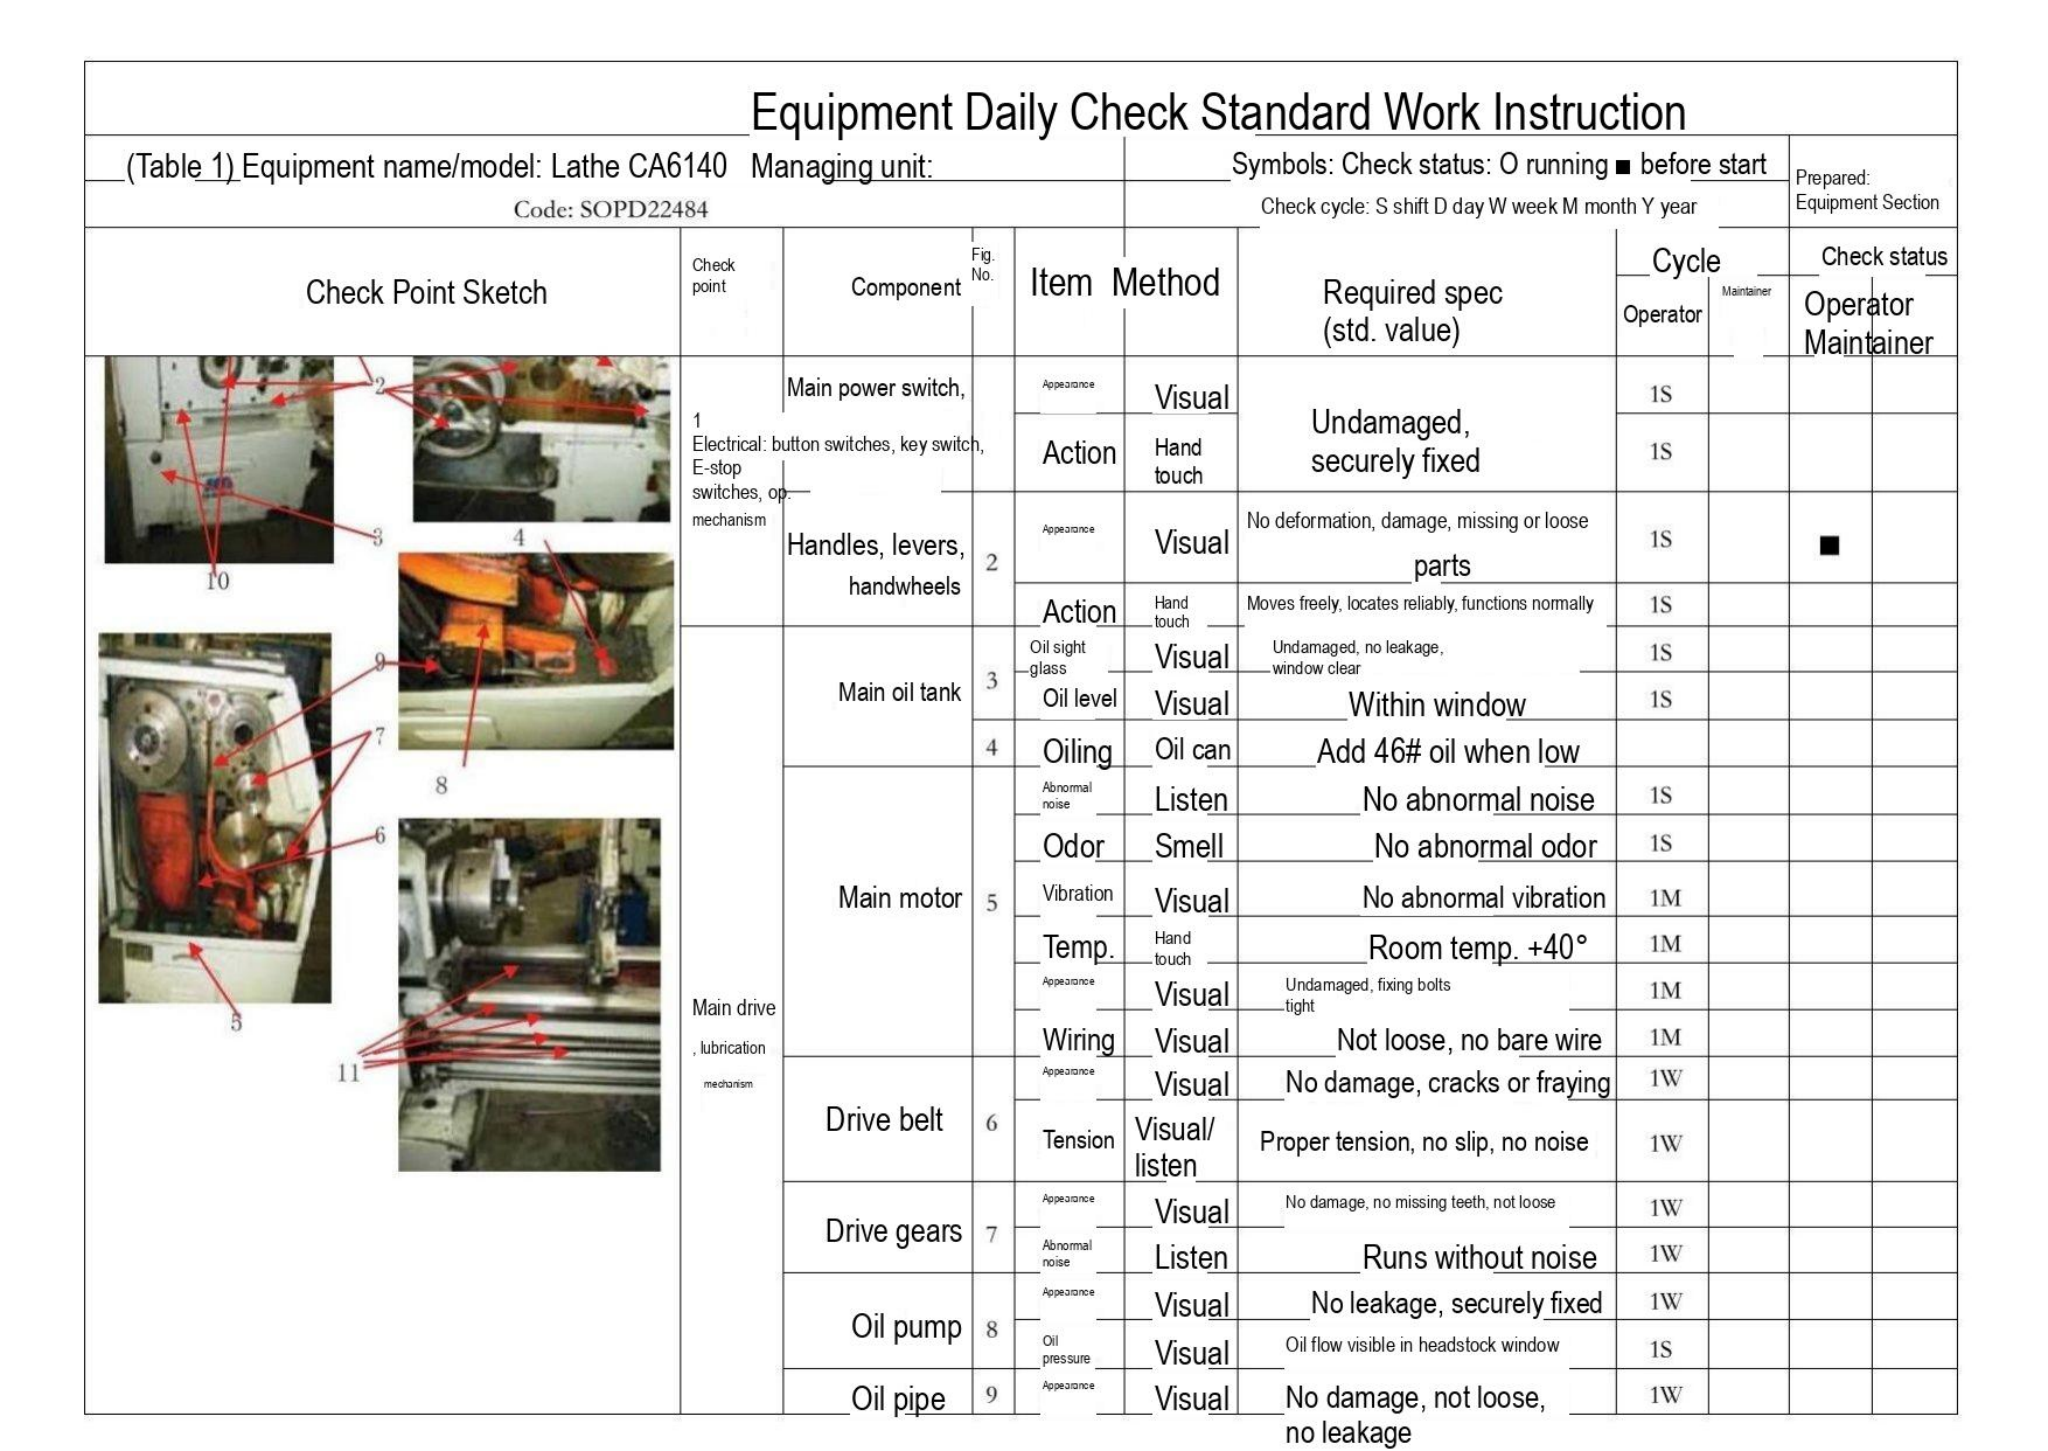# Equipment Daily Check Standard Work Instruction

(Table 1) Equipment name/model: Lathe CA6140 Managing unit:

Code: SOPD22484

Symbols: Check status: O running ■ before start

Check cycle: S shift D day W week M month Y year

Prepared: Equipment Section

Check Point Sketch

2 4 3 10 9 7 8 6 5 11

| Check point | Component | Fig. No. | Item | Method | Required spec (std. value) | Cycle Operator | Cycle Maintainer | Check status Operator | Check status Maintainer |
|---|---|---|---|---|---|---|---|---|---|
| 1 Electrical: button switches, key switch, E-stop switches, op. mechanism | Main power switch, | | Appearance | Visual | Undamaged, securely fixed | 1S | | | |
| | | | Action | Hand touch | | 1S | | | |
| | Handles, levers, handwheels | 2 | Appearance | Visual | No deformation, damage, missing or loose parts | 1S | | ■ | |
| | | | Action | Hand touch | Moves freely, locates reliably, functions normally | 1S | | | |
| Main drive, lubrication mechanism | Main oil tank | 3 | Oil sight glass | Visual | Undamaged, no leakage, window clear | 1S | | | |
| | | | Oil level | Visual | Within window | 1S | | | |
| | | 4 | Oiling | Oil can | Add 46# oil when low | | | | |
| | Main motor | 5 | Abnormal noise | Listen | No abnormal noise | 1S | | | |
| | | | Odor | Smell | No abnormal odor | 1S | | | |
| | | | Vibration | Visual | No abnormal vibration | 1M | | | |
| | | | Temp. | Hand touch | Room temp. +40° | 1M | | | |
| | | | Appearance | Visual | Undamaged, fixing bolts tight | 1M | | | |
| | | | Wiring | Visual | Not loose, no bare wire | 1M | | | |
| | Drive belt | 6 | Appearance | Visual | No damage, cracks or fraying | 1W | | | |
| | | | Tension | Visual/ listen | Proper tension, no slip, no noise | 1W | | | |
| | Drive gears | 7 | Appearance | Visual | No damage, no missing teeth, not loose | 1W | | | |
| | | | Abnormal noise | Listen | Runs without noise | 1W | | | |
| | Oil pump | 8 | Appearance | Visual | No leakage, securely fixed | 1W | | | |
| | | | Oil pressure | Visual | Oil flow visible in headstock window | 1S | | | |
| | Oil pipe | 9 | Appearance | Visual | No damage, not loose, no leakage | 1W | | | |
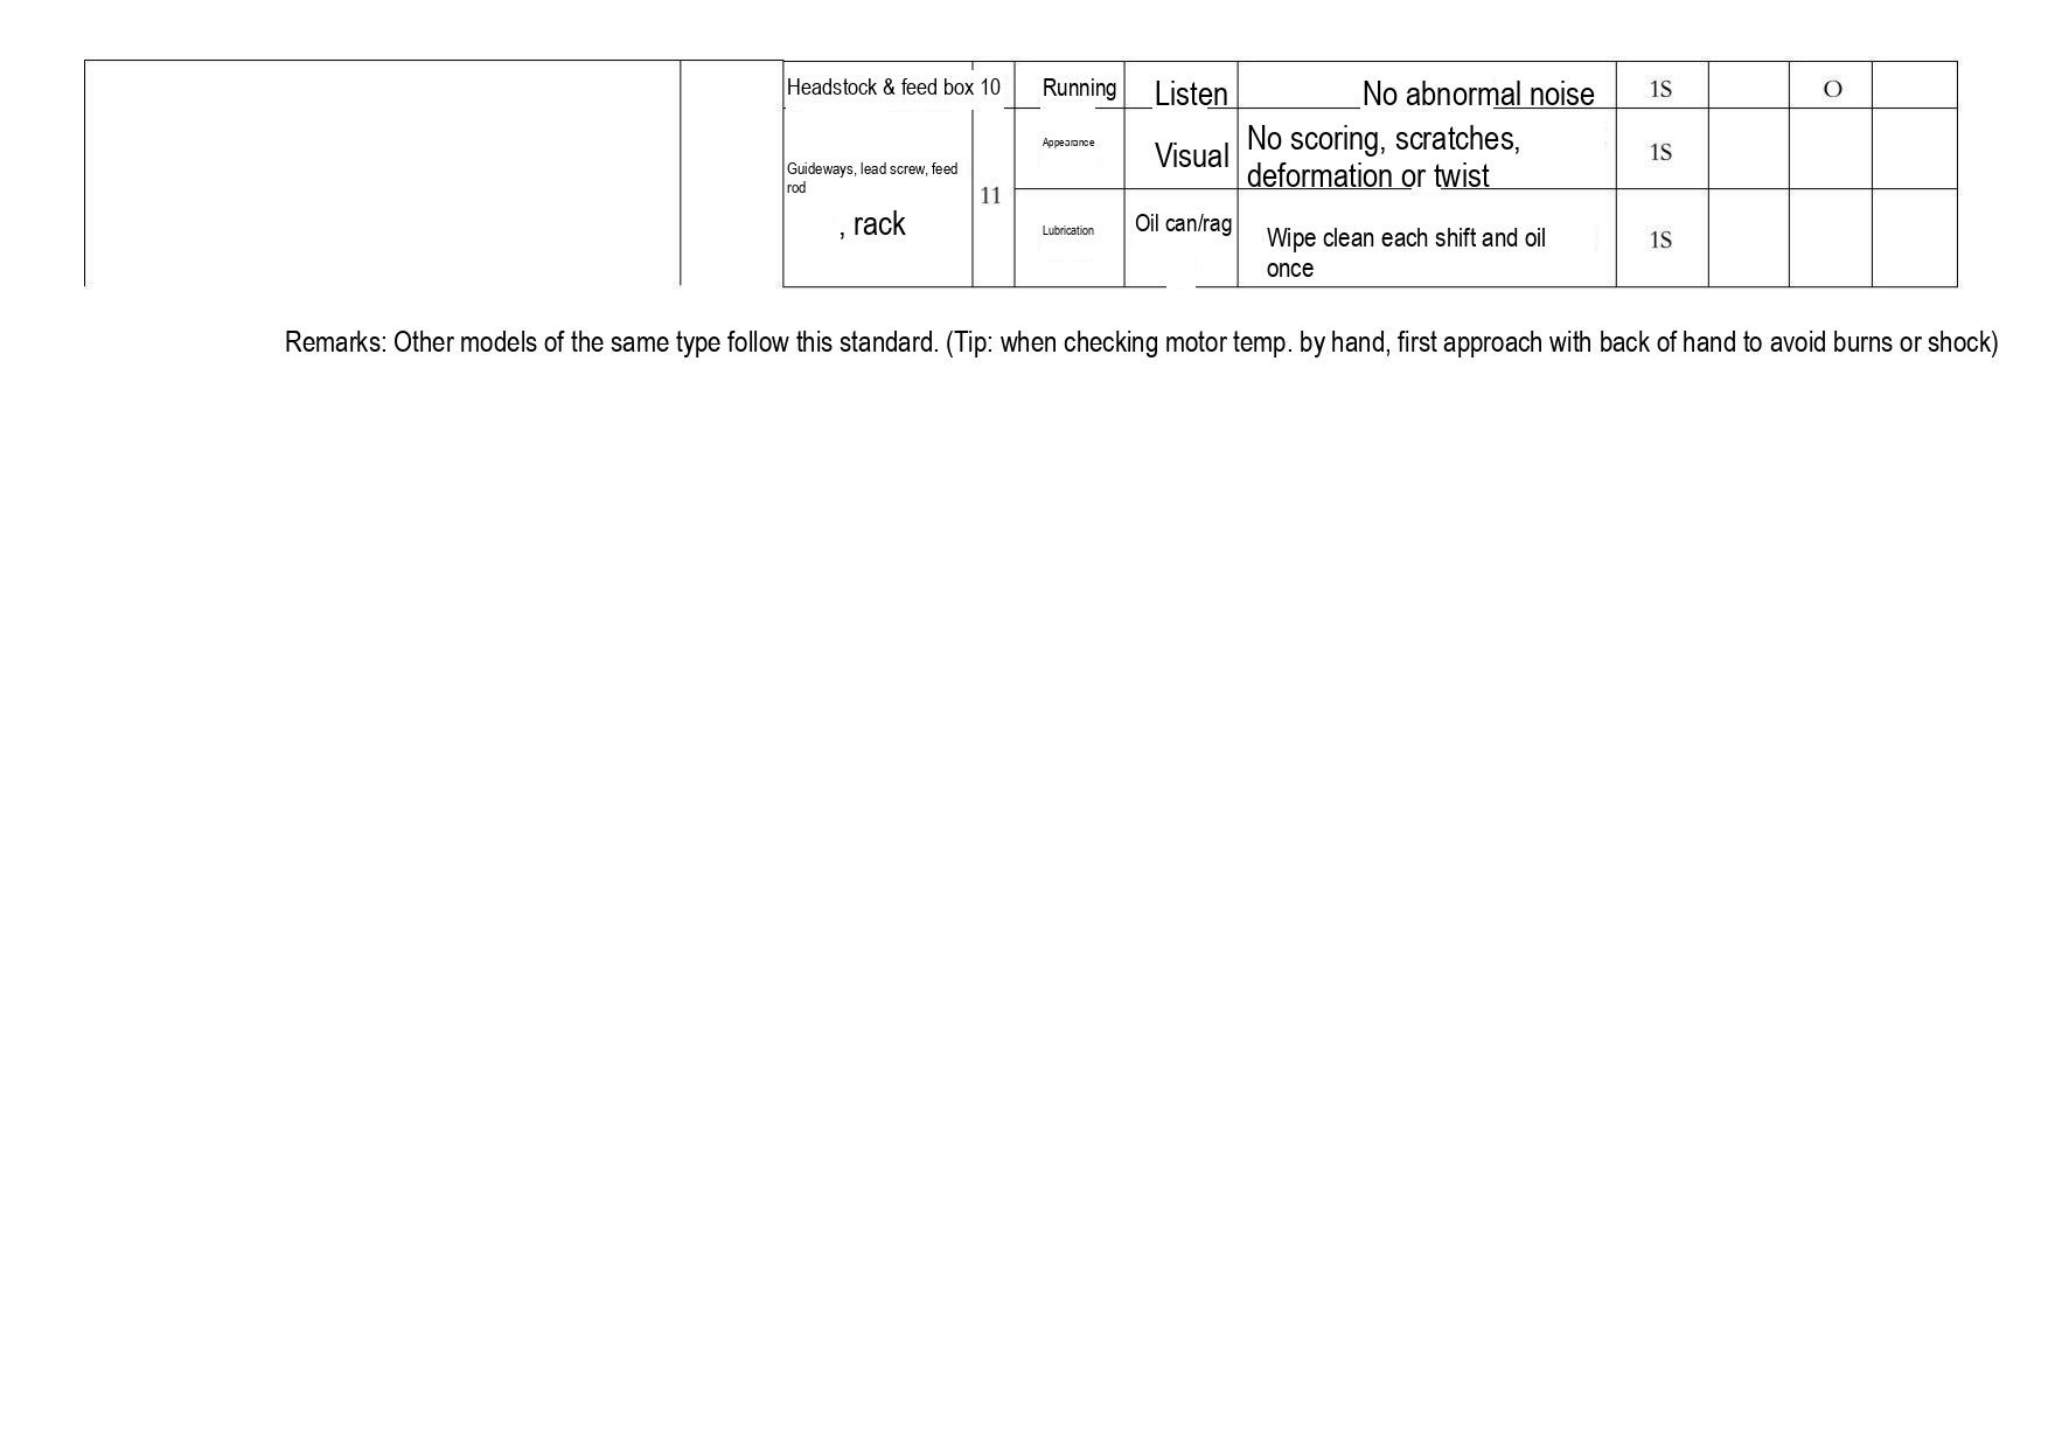| | | | | | | | | | | |
|---|---|---|---|---|---|---|---|---|---|---|
| | | Headstock & feed box | 10 | Running | Listen | No abnormal noise | 1S | | O | |
| | | Guideways, lead screw, feed rod , rack | 11 | Appearance | Visual | No scoring, scratches, deformation or twist | 1S | | | |
| | | | | Lubrication | Oil can/rag | Wipe clean each shift and oil once | 1S | | | |

Remarks: Other models of the same type follow this standard. (Tip: when checking motor temp. by hand, first approach with back of hand to avoid burns or shock)
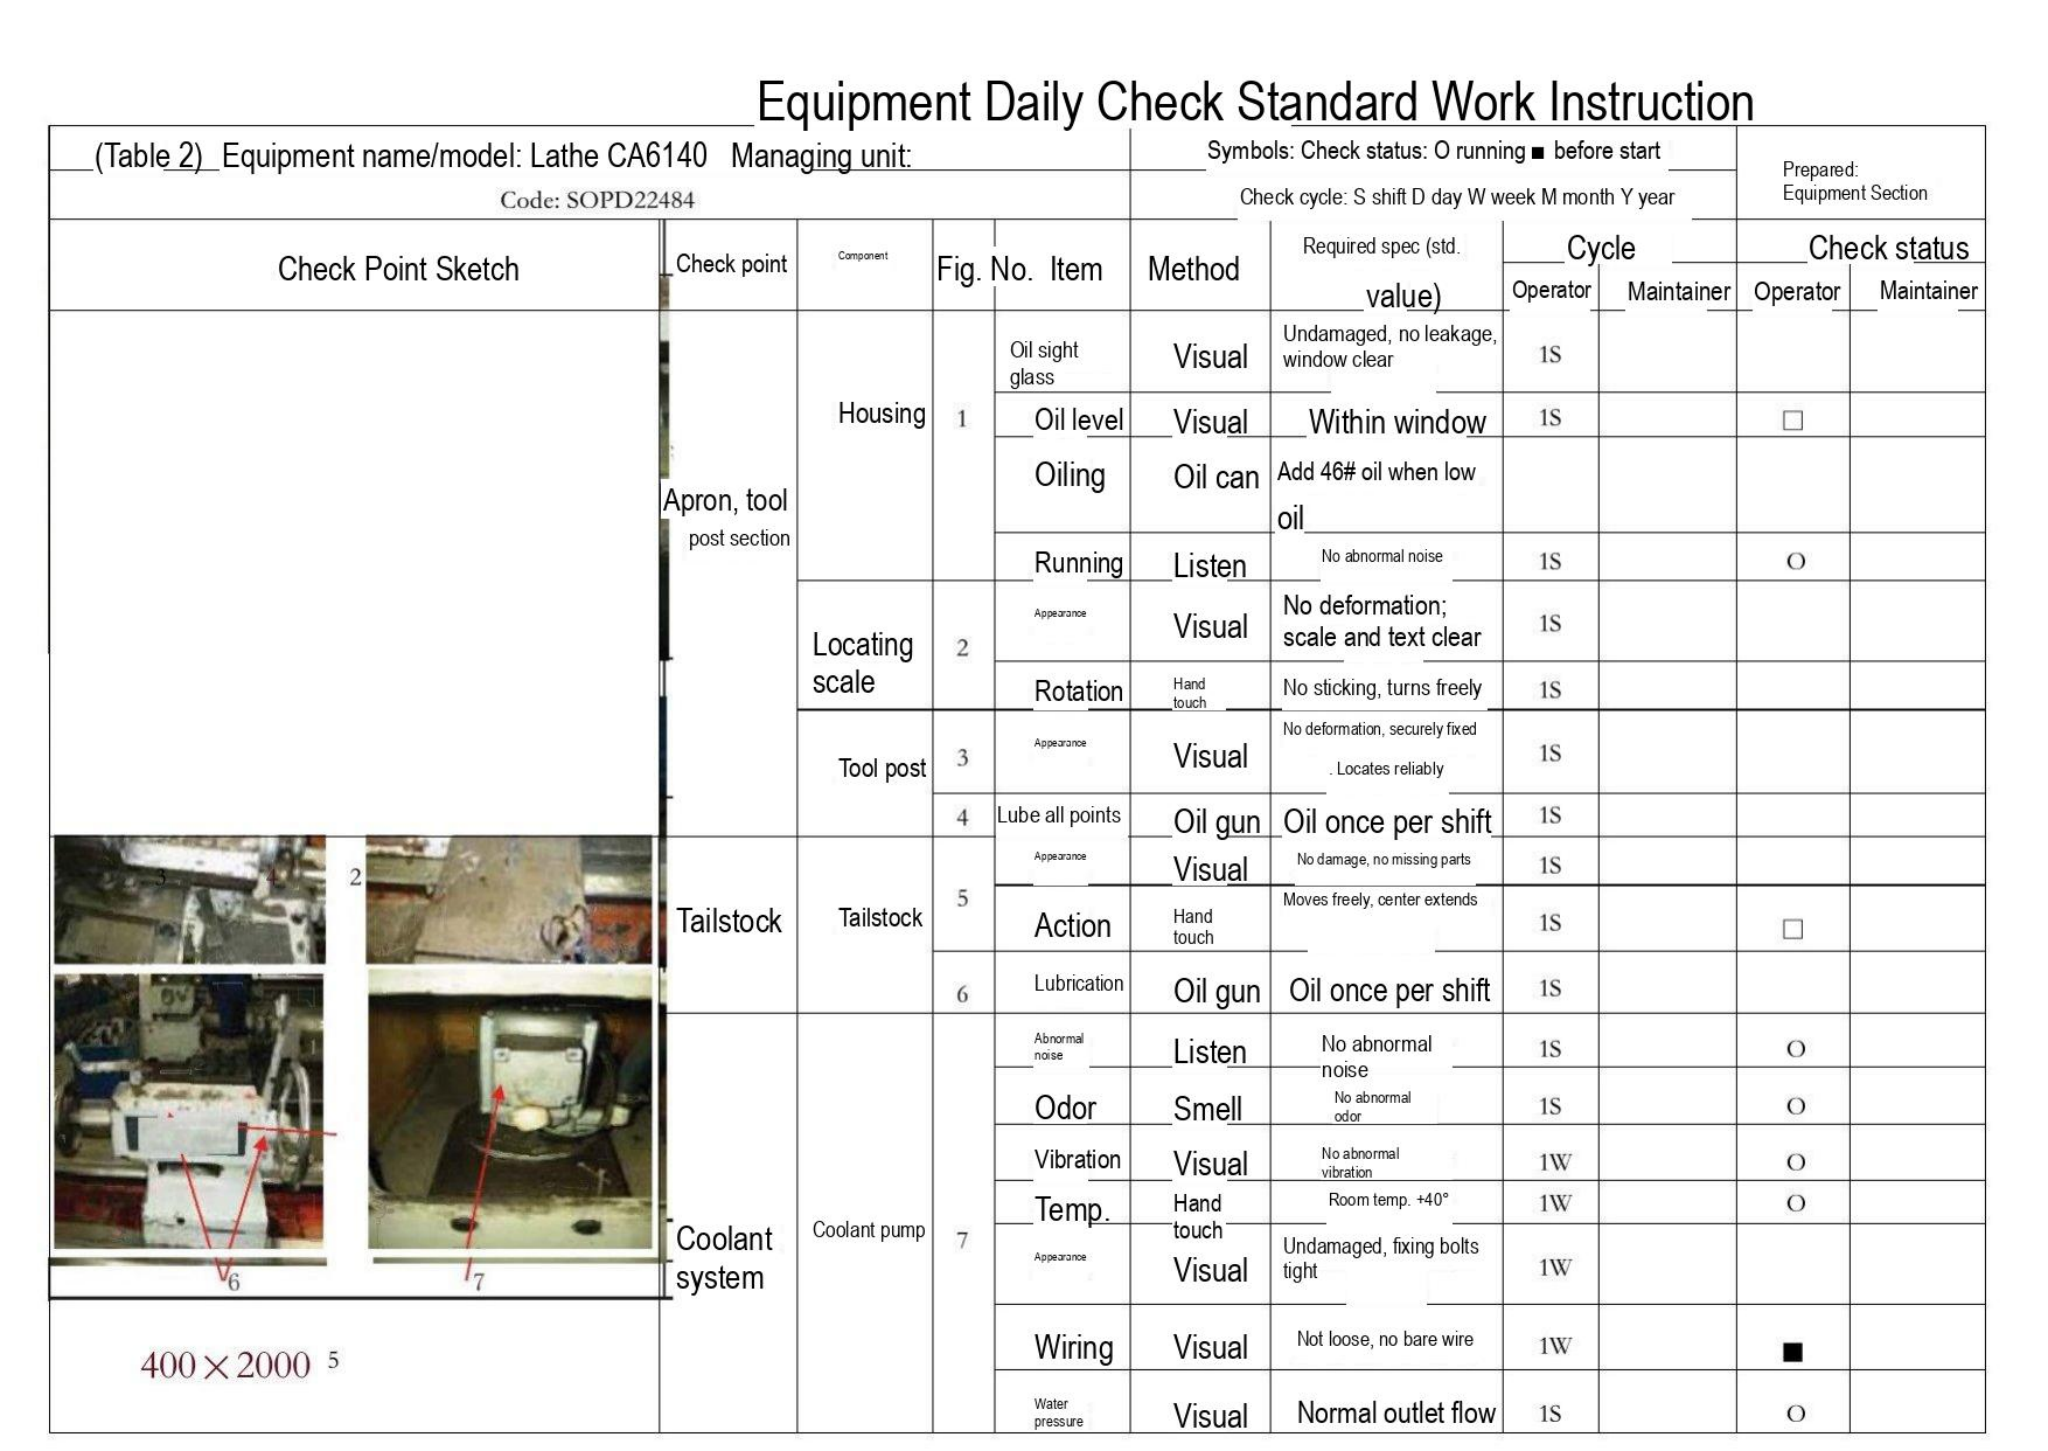# Equipment Daily Check Standard Work Instruction

(Table 2) Equipment name/model: Lathe CA6140 Managing unit:

Code: SOPD22484

Symbols: Check status: O running ■ before start

Check cycle: S shift D day W week M month Y year

Prepared: Equipment Section

Check Point Sketch

3 4 2

6 7

400 × 2000 5

| Check point | Component | Fig. No. | Item | Method | Required spec (std. value) | Cycle: Operator | Cycle: Maintainer | Check status: Operator | Check status: Maintainer |
|---|---|---|---|---|---|---|---|---|---|
| Apron, tool post section | Housing | 1 | Oil sight glass | Visual | Undamaged, no leakage, window clear | 1S | | | |
| | | | Oil level | Visual | Within window | 1S | | □ | |
| | | | Oiling | Oil can | Add 46# oil when low oil | | | | |
| | | | Running | Listen | No abnormal noise | 1S | | O | |
| | Locating scale | 2 | Appearance | Visual | No deformation; scale and text clear | 1S | | | |
| | | | Rotation | Hand touch | No sticking, turns freely | 1S | | | |
| | Tool post | 3 | Appearance | Visual | No deformation, securely fixed . Locates reliably | 1S | | | |
| | | 4 | Lube all points | Oil gun | Oil once per shift | 1S | | | |
| Tailstock | Tailstock | 5 | Appearance | Visual | No damage, no missing parts | 1S | | | |
| | | | Action | Hand touch | Moves freely, center extends | 1S | | □ | |
| | | 6 | Lubrication | Oil gun | Oil once per shift | 1S | | | |
| Coolant system | Coolant pump | 7 | Abnormal noise | Listen | No abnormal noise | 1S | | O | |
| | | | Odor | Smell | No abnormal odor | 1S | | O | |
| | | | Vibration | Visual | No abnormal vibration | 1W | | O | |
| | | | Temp. | Hand touch | Room temp. +40° | 1W | | O | |
| | | | Appearance | Visual | Undamaged, fixing bolts tight | 1W | | | |
| | | | Wiring | Visual | Not loose, no bare wire | 1W | | ■ | |
| | | | Water pressure | Visual | Normal outlet flow | 1S | | O | |
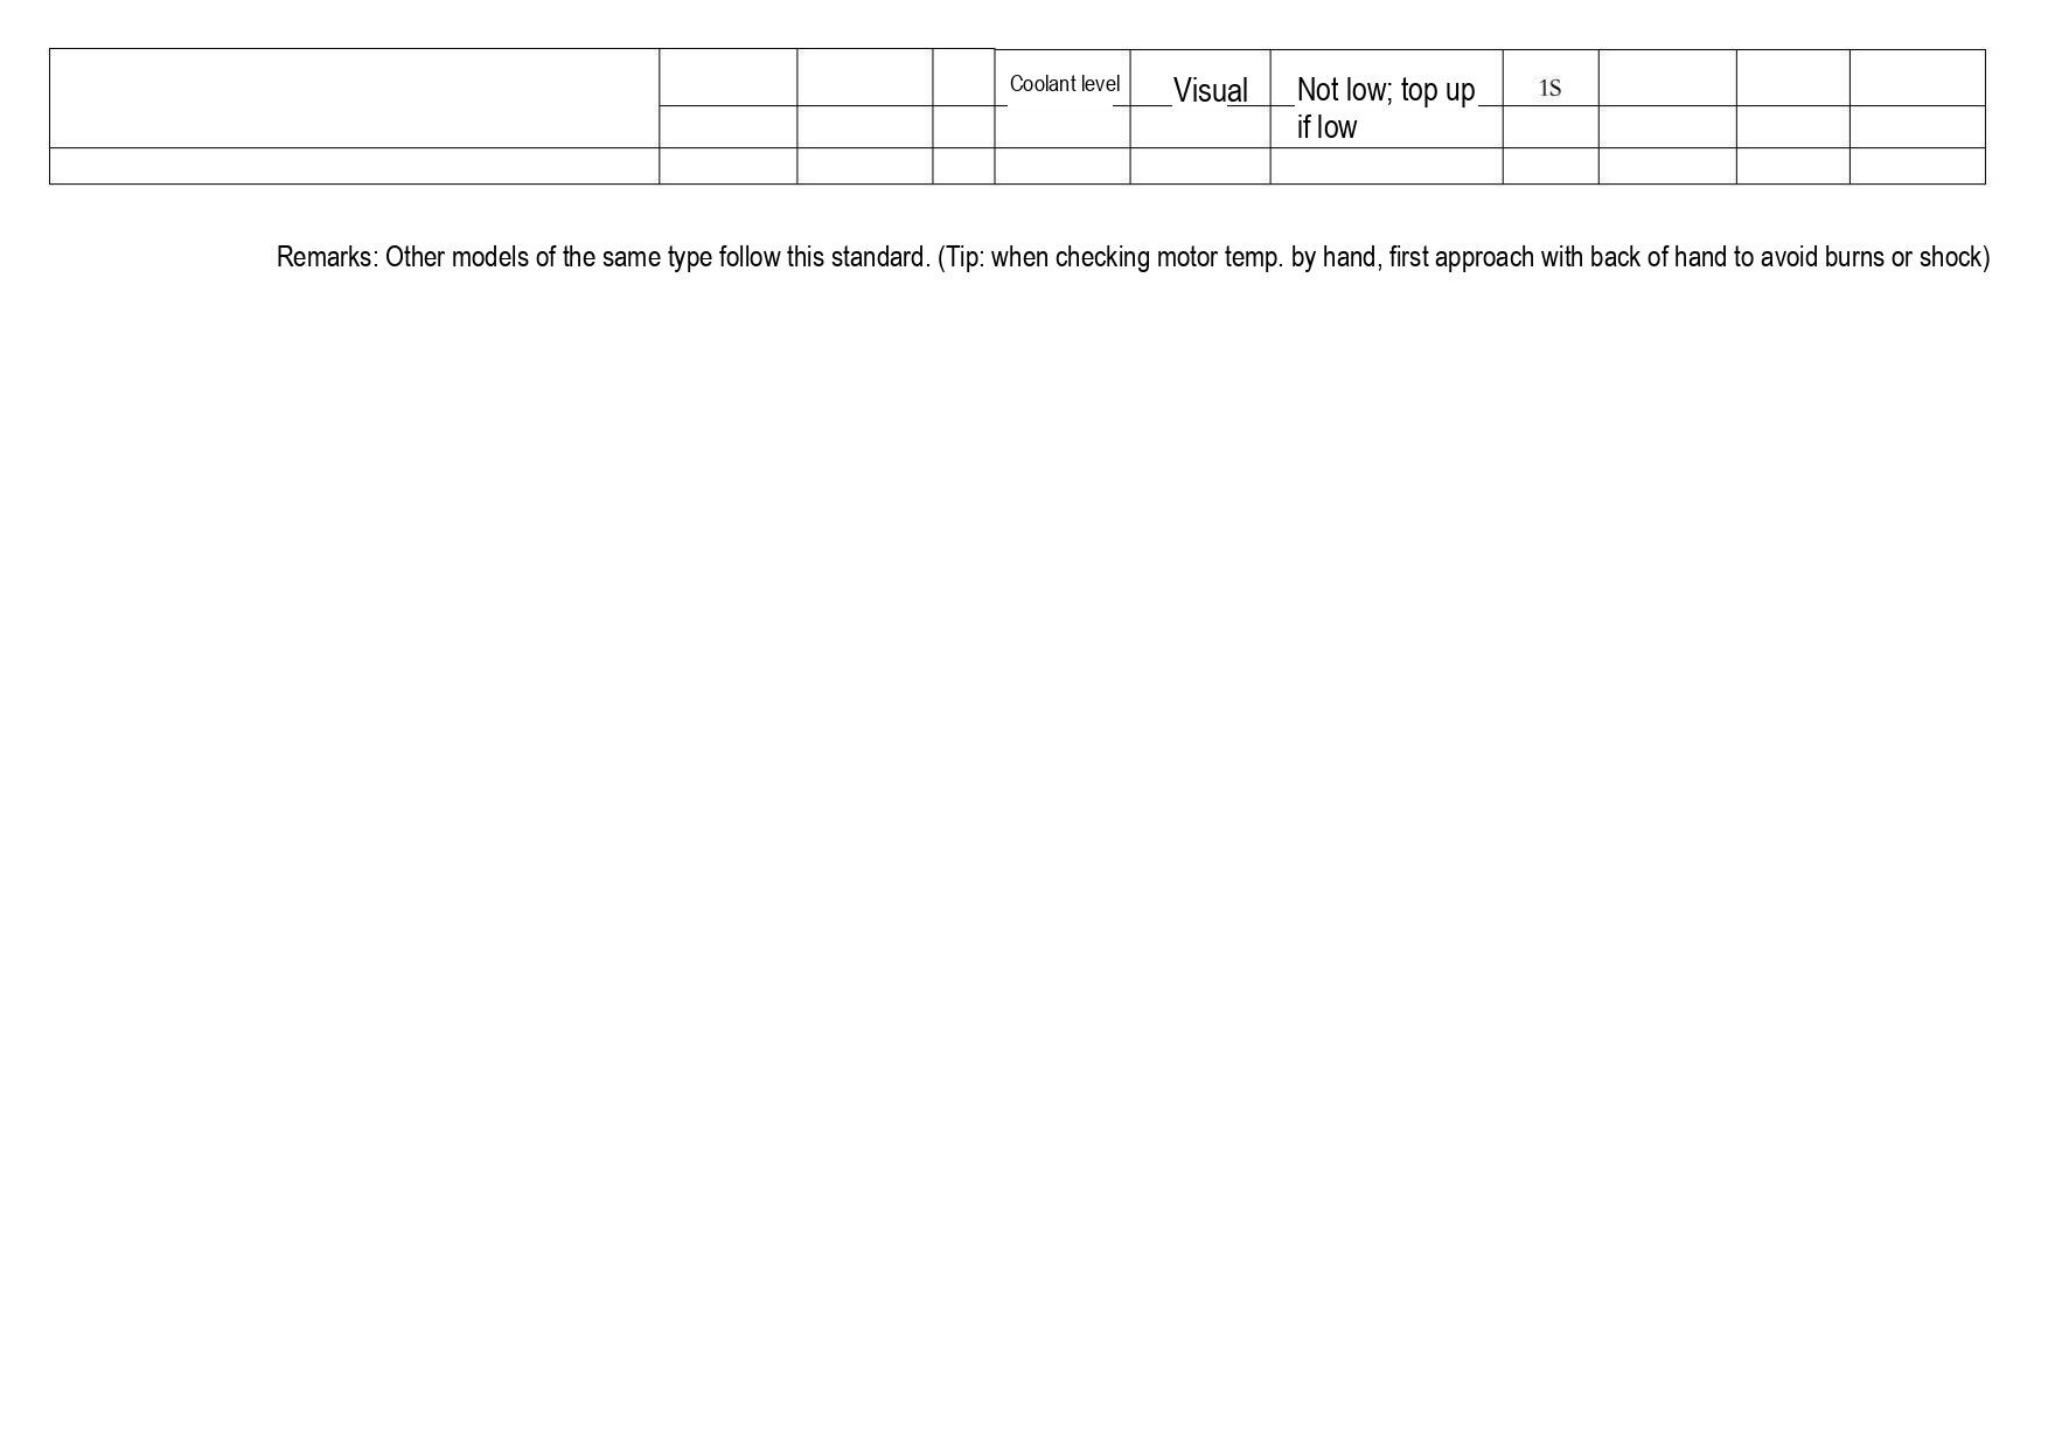|  |  |  |  | Coolant level | Visual | Not low; top up if low | 1S |  |  |  |
|---|---|---|---|---|---|---|---|---|---|---|
|  |  |  |  |  |  |  |  |  |  |  |

Remarks: Other models of the same type follow this standard. (Tip: when checking motor temp. by hand, first approach with back of hand to avoid burns or shock)